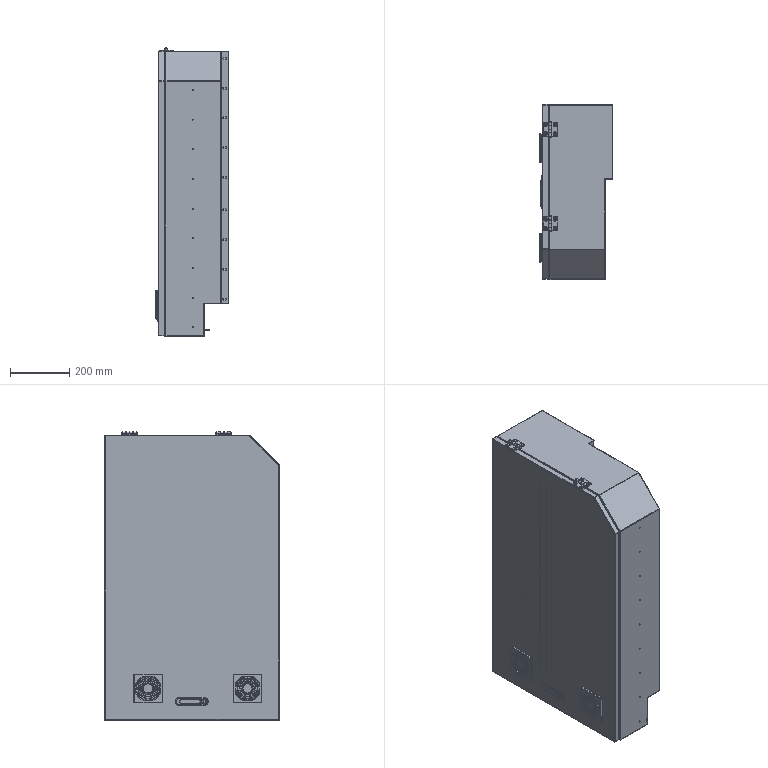Part | SolidWorks | features InContextFeatHolder 11, ReferencePattern 7, LocalLPattern 1 | 36 solids | 4180 faces | volume 8213820 mm3 | plane 2441 | cylinder 1175 | torus 328 | cone 109 | spline 101 | sphere 26 | commonest cylinder face diameters 3.3 x136 1 x126 2 x98 5 x82 7 x64 8 x52